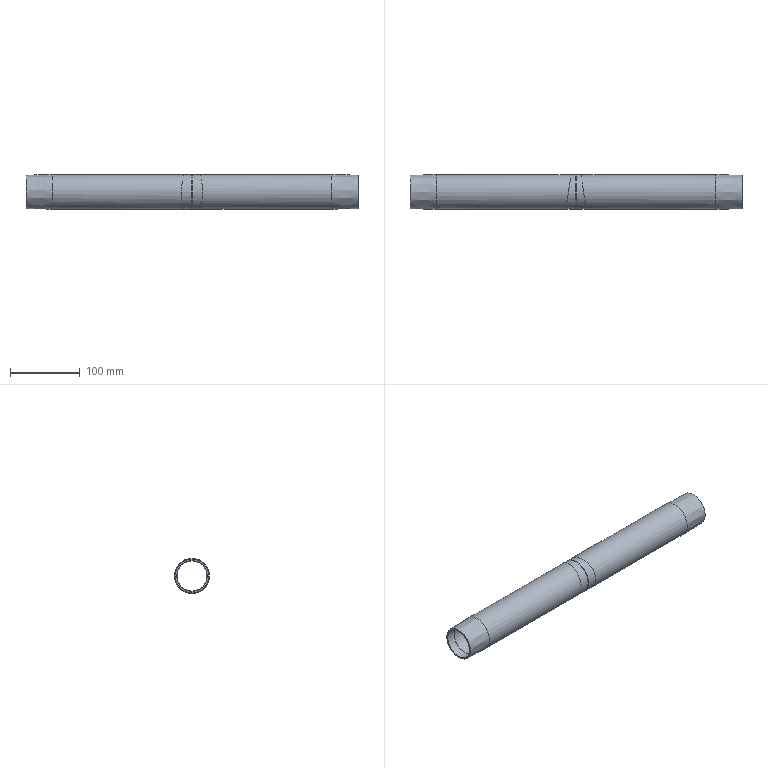Part | STEP file | 6150801 | 1 solid | 14 faces | box 475 x 50 x 50 mm | volume 235448 mm3 | cylinder 8 | plane 4 | cone 2 | commonest cylinder face diameters 50 x5 44 x2 43 x1
STEP:
#1=CARTESIAN_POINT('',(-0.5,-25.,0.));
#2=VERTEX_POINT('',#1);
#3=CARTESIAN_POINT('',(-0.5,0.,0.));
#4=DIRECTION('',(-1.,0.,0.));
#5=DIRECTION('',(0.,-1.,0.));
#6=AXIS2_PLACEMENT_3D('',#3,#4,#5);
#7=CIRCLE('',#6,25.);
#8=EDGE_CURVE('',#2,#2,#7,.T.);
#9=ORIENTED_EDGE('',*,*,#8,.F.);
#10=EDGE_LOOP('',(#9));
#11=FACE_OUTER_BOUND('',#10,.T.);
#12=CARTESIAN_POINT('',(0.5,25.,0.));
#13=VERTEX_POINT('',#12);
#14=CARTESIAN_POINT('',(0.5,0.,0.));
#15=DIRECTION('',(1.,0.,0.));
#16=DIRECTION('',(0.,1.,0.));
#17=AXIS2_PLACEMENT_3D('',#14,#15,#16);
#18=CIRCLE('',#17,25.);
#19=EDGE_CURVE('',#13,#13,#18,.T.);
#20=ORIENTED_EDGE('',*,*,#19,.F.);
#21=EDGE_LOOP('',(#20));
#22=FACE_OUTER_BOUND('',#21,.T.);
#23=CARTESIAN_POINT('',(-73.378,0.,0.));
#24=DIRECTION('',(-1.,0.,0.));
#25=DIRECTION('',(0.,0.,1.));
#26=AXIS2_PLACEMENT_3D('',#23,#24,#25);
#27=CYLINDRICAL_SURFACE('',#26,25.);
#28=ADVANCED_FACE('',(#11,#22),#27,.T.);
#29=CARTESIAN_POINT('',(200.,0.,25.));
#30=VERTEX_POINT('',#29);
#31=CARTESIAN_POINT('',(200.,0.,0.));
#32=DIRECTION('',(-1.,0.,0.));
#33=DIRECTION('',(0.,0.,1.));
#34=AXIS2_PLACEMENT_3D('',#31,#32,#33);
#35=CIRCLE('',#34,25.);
#36=EDGE_CURVE('',#30,#30,#35,.T.);
#37=ORIENTED_EDGE('',*,*,#36,.T.);
#38=EDGE_LOOP('',(#37));
#39=FACE_OUTER_BOUND('',#38,.T.);
#40=CARTESIAN_POINT('',(7.038,25.,0.));
#41=VERTEX_POINT('',#40);
#42=CARTESIAN_POINT('',(7.038,25.,0.));
#43=CARTESIAN_POINT('',(7.038,25.,-50.));
#44=CARTESIAN_POINT('',(14.731,-25.,-50.));
#45=CARTESIAN_POINT('',(14.731,-25.,0.));
#46=CARTESIAN_POINT('',(14.731,-25.,50.));
#47=CARTESIAN_POINT('',(7.038,25.,50.));
#48=CARTESIAN_POINT('',(7.038,25.,0.));
#49=(BOUNDED_CURVE()B_SPLINE_CURVE(3,(#42,#43,#44,#45,#46,#47,#48),.UNSPECIFIED.,.T.,.T.)B_SPLINE_CURVE_WITH_KNOTS((4,3,4),(0.,3.142,6.283),.UNSPECIFIED.)CURVE()GEOMETRIC_REPRESENTATION_ITEM()RATIONAL_B_SPLINE_CURVE((1.,0.3333,0.3333,1.,0.3333,0.3333,1.))REPRESENTATION_ITEM(''));
#50=EDGE_CURVE('',#41,#41,#49,.T.);
#51=ORIENTED_EDGE('',*,*,#50,.F.);
#52=EDGE_LOOP('',(#51));
#53=FACE_OUTER_BOUND('',#52,.T.);
#54=CARTESIAN_POINT('',(-73.378,0.,0.));
#55=DIRECTION('',(-1.,0.,0.));
#56=DIRECTION('',(0.,0.,1.));
#57=AXIS2_PLACEMENT_3D('',#54,#55,#56);
#58=CYLINDRICAL_SURFACE('',#57,25.);
#59=ADVANCED_FACE('',(#39,#53),#58,.T.);
#60=CARTESIAN_POINT('',(-200.,0.,25.));
#61=VERTEX_POINT('',#60);
#62=CARTESIAN_POINT('',(-200.,0.,0.));
#63=DIRECTION('',(-1.,0.,0.));
#64=DIRECTION('',(0.,0.,1.));
#65=AXIS2_PLACEMENT_3D('',#62,#63,#64);
#66=CIRCLE('',#65,25.);
#67=EDGE_CURVE('',#61,#61,#66,.T.);
#68=ORIENTED_EDGE('',*,*,#67,.F.);
#69=EDGE_LOOP('',(#68));
#70=FACE_OUTER_BOUND('',#69,.T.);
#71=CARTESIAN_POINT('',(-14.731,-25.,0.));
#72=VERTEX_POINT('',#71);
#73=CARTESIAN_POINT('',(-14.731,-25.,0.));
#74=CARTESIAN_POINT('',(-14.731,-25.,-50.));
#75=CARTESIAN_POINT('',(-7.038,25.,-50.));
#76=CARTESIAN_POINT('',(-7.038,25.,0.));
#77=CARTESIAN_POINT('',(-7.038,25.,50.));
#78=CARTESIAN_POINT('',(-14.731,-25.,50.));
#79=CARTESIAN_POINT('',(-14.731,-25.,0.));
#80=(BOUNDED_CURVE()B_SPLINE_CURVE(3,(#73,#74,#75,#76,#77,#78,#79),.UNSPECIFIED.,.T.,.F.)B_SPLINE_CURVE_WITH_KNOTS((4,3,4),(0.,3.142,6.283),.UNSPECIFIED.)CURVE()GEOMETRIC_REPRESENTATION_ITEM()RATIONAL_B_SPLINE_CURVE((1.,0.3333,0.3333,1.,0.3333,0.3333,1.))REPRESENTATION_ITEM(''));
#81=EDGE_CURVE('',#72,#72,#80,.T.);
#82=ORIENTED_EDGE('',*,*,#81,.F.);
#83=EDGE_LOOP('',(#82));
#84=FACE_OUTER_BOUND('',#83,.T.);
#85=CARTESIAN_POINT('',(-73.378,0.,0.));
#86=DIRECTION('',(-1.,0.,0.));
#87=DIRECTION('',(0.,0.,1.));
#88=AXIS2_PLACEMENT_3D('',#85,#86,#87);
#89=CYLINDRICAL_SURFACE('',#88,25.);
#90=ADVANCED_FACE('',(#70,#84),#89,.T.);
#91=ORIENTED_EDGE('',*,*,#19,.T.);
#92=EDGE_LOOP('',(#91));
#93=FACE_OUTER_BOUND('',#92,.T.);
#94=ORIENTED_EDGE('',*,*,#50,.T.);
#95=EDGE_LOOP('',(#94));
#96=FACE_OUTER_BOUND('',#95,.T.);
#97=CARTESIAN_POINT('',(-73.378,0.,0.));
#98=DIRECTION('',(-1.,0.,0.));
#99=DIRECTION('',(0.,0.,1.));
#100=AXIS2_PLACEMENT_3D('',#97,#98,#99);
#101=CYLINDRICAL_SURFACE('',#100,25.);
#102=ADVANCED_FACE('',(#93,#96),#101,.T.);
#103=CARTESIAN_POINT('',(237.5,0.,24.018));
#104=VERTEX_POINT('',#103);
#105=CARTESIAN_POINT('',(237.5,0.,0.));
#106=DIRECTION('',(-1.,0.,0.));
#107=DIRECTION('',(0.,0.,1.));
#108=AXIS2_PLACEMENT_3D('',#105,#106,#107);
#109=CIRCLE('',#108,24.018);
#110=EDGE_CURVE('',#104,#104,#109,.T.);
#111=ORIENTED_EDGE('',*,*,#110,.F.);
#112=EDGE_LOOP('',(#111));
#113=FACE_OUTER_BOUND('',#112,.T.);
#114=CARTESIAN_POINT('',(237.5,0.,22.));
#115=VERTEX_POINT('',#114);
#116=CARTESIAN_POINT('',(237.5,0.,0.));
#117=DIRECTION('',(-1.,0.,0.));
#118=DIRECTION('',(0.,0.,1.));
#119=AXIS2_PLACEMENT_3D('',#116,#117,#118);
#120=CIRCLE('',#119,22.);
#121=EDGE_CURVE('',#115,#115,#120,.T.);
#122=ORIENTED_EDGE('',*,*,#121,.T.);
#123=EDGE_LOOP('',(#122));
#124=FACE_BOUND('',#123,.T.);
#125=CARTESIAN_POINT('',(237.5,24.018,0.));
#126=DIRECTION('',(-1.,0.,0.));
#127=DIRECTION('',(0.,0.,1.));
#128=AXIS2_PLACEMENT_3D('',#125,#126,#127);
#129=PLANE('',#128);
#130=ADVANCED_FACE('',(#113,#124),#129,.F.);
#131=ORIENTED_EDGE('',*,*,#121,.F.);
#132=EDGE_LOOP('',(#131));
#133=FACE_OUTER_BOUND('',#132,.T.);
#134=CARTESIAN_POINT('',(225.,0.,22.));
#135=VERTEX_POINT('',#134);
#136=CARTESIAN_POINT('',(225.,0.,0.));
#137=DIRECTION('',(-1.,0.,0.));
#138=DIRECTION('',(0.,0.,1.));
#139=AXIS2_PLACEMENT_3D('',#136,#137,#138);
#140=CIRCLE('',#139,22.);
#141=EDGE_CURVE('',#135,#135,#140,.T.);
#142=ORIENTED_EDGE('',*,*,#141,.T.);
#143=EDGE_LOOP('',(#142));
#144=FACE_OUTER_BOUND('',#143,.T.);
#145=CARTESIAN_POINT('',(-73.378,0.,0.));
#146=DIRECTION('',(-1.,0.,0.));
#147=DIRECTION('',(0.,0.,1.));
#148=AXIS2_PLACEMENT_3D('',#145,#146,#147);
#149=CYLINDRICAL_SURFACE('',#148,22.);
#150=ADVANCED_FACE('',(#133,#144),#149,.F.);
#151=ORIENTED_EDGE('',*,*,#141,.F.);
#152=EDGE_LOOP('',(#151));
#153=FACE_OUTER_BOUND('',#152,.T.);
#154=CARTESIAN_POINT('',(225.,0.,21.5));
#155=VERTEX_POINT('',#154);
#156=CARTESIAN_POINT('',(225.,0.,0.));
#157=DIRECTION('',(-1.,0.,0.));
#158=DIRECTION('',(0.,0.,1.));
#159=AXIS2_PLACEMENT_3D('',#156,#157,#158);
#160=CIRCLE('',#159,21.5);
#161=EDGE_CURVE('',#155,#155,#160,.T.);
#162=ORIENTED_EDGE('',*,*,#161,.T.);
#163=EDGE_LOOP('',(#162));
#164=FACE_BOUND('',#163,.T.);
#165=CARTESIAN_POINT('',(225.,22.,0.));
#166=DIRECTION('',(-1.,0.,0.));
#167=DIRECTION('',(0.,0.,1.));
#168=AXIS2_PLACEMENT_3D('',#165,#166,#167);
#169=PLANE('',#168);
#170=ADVANCED_FACE('',(#153,#164),#169,.F.);
#171=ORIENTED_EDGE('',*,*,#161,.F.);
#172=EDGE_LOOP('',(#171));
#173=FACE_OUTER_BOUND('',#172,.T.);
#174=CARTESIAN_POINT('',(-225.,0.,21.5));
#175=VERTEX_POINT('',#174);
#176=CARTESIAN_POINT('',(-225.,0.,0.));
#177=DIRECTION('',(-1.,0.,0.));
#178=DIRECTION('',(0.,0.,1.));
#179=AXIS2_PLACEMENT_3D('',#176,#177,#178);
#180=CIRCLE('',#179,21.5);
#181=EDGE_CURVE('',#175,#175,#180,.T.);
#182=ORIENTED_EDGE('',*,*,#181,.T.);
#183=EDGE_LOOP('',(#182));
#184=FACE_OUTER_BOUND('',#183,.T.);
#185=CARTESIAN_POINT('',(-73.378,0.,0.));
#186=DIRECTION('',(-1.,0.,0.));
#187=DIRECTION('',(0.,0.,1.));
#188=AXIS2_PLACEMENT_3D('',#185,#186,#187);
#189=CYLINDRICAL_SURFACE('',#188,21.5);
#190=ADVANCED_FACE('',(#173,#184),#189,.F.);
#191=ORIENTED_EDGE('',*,*,#181,.F.);
#192=EDGE_LOOP('',(#191));
#193=FACE_BOUND('',#192,.T.);
#194=CARTESIAN_POINT('',(-225.,0.,22.));
#195=VERTEX_POINT('',#194);
#196=CARTESIAN_POINT('',(-225.,0.,0.));
#197=DIRECTION('',(-1.,0.,0.));
#198=DIRECTION('',(0.,0.,1.));
#199=AXIS2_PLACEMENT_3D('',#196,#197,#198);
#200=CIRCLE('',#199,22.);
#201=EDGE_CURVE('',#195,#195,#200,.T.);
#202=ORIENTED_EDGE('',*,*,#201,.T.);
#203=EDGE_LOOP('',(#202));
#204=FACE_OUTER_BOUND('',#203,.T.);
#205=CARTESIAN_POINT('',(-225.,22.,0.));
#206=DIRECTION('',(1.,0.,0.));
#207=DIRECTION('',(0.,0.,-1.));
#208=AXIS2_PLACEMENT_3D('',#205,#206,#207);
#209=PLANE('',#208);
#210=ADVANCED_FACE('',(#193,#204),#209,.F.);
#211=ORIENTED_EDGE('',*,*,#201,.F.);
#212=EDGE_LOOP('',(#211));
#213=FACE_OUTER_BOUND('',#212,.T.);
#214=CARTESIAN_POINT('',(-237.5,0.,22.));
#215=VERTEX_POINT('',#214);
#216=CARTESIAN_POINT('',(-237.5,0.,0.));
#217=DIRECTION('',(-1.,0.,0.));
#218=DIRECTION('',(0.,0.,1.));
#219=AXIS2_PLACEMENT_3D('',#216,#217,#218);
#220=CIRCLE('',#219,22.);
#221=EDGE_CURVE('',#215,#215,#220,.T.);
#222=ORIENTED_EDGE('',*,*,#221,.T.);
#223=EDGE_LOOP('',(#222));
#224=FACE_OUTER_BOUND('',#223,.T.);
#225=CARTESIAN_POINT('',(-73.378,0.,0.));
#226=DIRECTION('',(-1.,0.,0.));
#227=DIRECTION('',(0.,0.,1.));
#228=AXIS2_PLACEMENT_3D('',#225,#226,#227);
#229=CYLINDRICAL_SURFACE('',#228,22.);
#230=ADVANCED_FACE('',(#213,#224),#229,.F.);
#231=ORIENTED_EDGE('',*,*,#221,.F.);
#232=EDGE_LOOP('',(#231));
#233=FACE_BOUND('',#232,.T.);
#234=CARTESIAN_POINT('',(-237.5,0.,24.018));
#235=VERTEX_POINT('',#234);
#236=CARTESIAN_POINT('',(-237.5,0.,0.));
#237=DIRECTION('',(-1.,0.,0.));
#238=DIRECTION('',(0.,0.,1.));
#239=AXIS2_PLACEMENT_3D('',#236,#237,#238);
#240=CIRCLE('',#239,24.018);
#241=EDGE_CURVE('',#235,#235,#240,.T.);
#242=ORIENTED_EDGE('',*,*,#241,.T.);
#243=EDGE_LOOP('',(#242));
#244=FACE_OUTER_BOUND('',#243,.T.);
#245=CARTESIAN_POINT('',(-237.5,22.,0.));
#246=DIRECTION('',(1.,0.,0.));
#247=DIRECTION('',(0.,0.,-1.));
#248=AXIS2_PLACEMENT_3D('',#245,#246,#247);
#249=PLANE('',#248);
#250=ADVANCED_FACE('',(#233,#244),#249,.F.);
#251=ORIENTED_EDGE('',*,*,#241,.F.);
#252=EDGE_LOOP('',(#251));
#253=FACE_BOUND('',#252,.T.);
#254=ORIENTED_EDGE('',*,*,#67,.T.);
#255=EDGE_LOOP('',(#254));
#256=FACE_OUTER_BOUND('',#255,.T.);
#257=CARTESIAN_POINT('',(-200.,0.,0.));
#258=DIRECTION('',(1.,0.,0.));
#259=DIRECTION('',(0.,0.,-1.));
#260=AXIS2_PLACEMENT_3D('',#257,#258,#259);
#261=CONICAL_SURFACE('',#260,25.,0.02618);
#262=ADVANCED_FACE('',(#253,#256),#261,.T.);
#263=ORIENTED_EDGE('',*,*,#81,.T.);
#264=EDGE_LOOP('',(#263));
#265=FACE_OUTER_BOUND('',#264,.T.);
#266=ORIENTED_EDGE('',*,*,#8,.T.);
#267=EDGE_LOOP('',(#266));
#268=FACE_OUTER_BOUND('',#267,.T.);
#269=CARTESIAN_POINT('',(-73.378,0.,0.));
#270=DIRECTION('',(-1.,0.,0.));
#271=DIRECTION('',(0.,0.,1.));
#272=AXIS2_PLACEMENT_3D('',#269,#270,#271);
#273=CYLINDRICAL_SURFACE('',#272,25.);
#274=ADVANCED_FACE('',(#265,#268),#273,.T.);
#275=ORIENTED_EDGE('',*,*,#36,.F.);
#276=EDGE_LOOP('',(#275));
#277=FACE_OUTER_BOUND('',#276,.T.);
#278=ORIENTED_EDGE('',*,*,#110,.T.);
#279=EDGE_LOOP('',(#278));
#280=FACE_BOUND('',#279,.T.);
#281=CARTESIAN_POINT('',(237.5,0.,0.));
#282=DIRECTION('',(-1.,0.,0.));
#283=DIRECTION('',(0.,0.,1.));
#284=AXIS2_PLACEMENT_3D('',#281,#282,#283);
#285=CONICAL_SURFACE('',#284,24.018,0.02618);
#286=ADVANCED_FACE('',(#277,#280),#285,.T.);
#287=CLOSED_SHELL('',(#28,#59,#90,#102,#130,#150,#170,#190,#210,#230,#250,#262,#274,#286));
#288=MANIFOLD_SOLID_BREP('',#287);
#289=CARTESIAN_POINT('',(0.,0.,0.));
#290=DIRECTION('',(0.,0.,1.));
#291=DIRECTION('',(1.,0.,0.));
#292=AXIS2_PLACEMENT_3D('',#289,#290,#291);
#293=(LENGTH_UNIT()NAMED_UNIT(*)SI_UNIT(.MILLI.,.METRE.));
#294=UNCERTAINTY_MEASURE_WITH_UNIT(LENGTH_MEASURE(0.00001),#293,'','');
#295=(NAMED_UNIT(*)PLANE_ANGLE_UNIT()SI_UNIT($,.RADIAN.));
#296=(NAMED_UNIT(*)SI_UNIT($,.STERADIAN.)SOLID_ANGLE_UNIT());
#297=(GEOMETRIC_REPRESENTATION_CONTEXT(3)GLOBAL_UNCERTAINTY_ASSIGNED_CONTEXT((#294))GLOBAL_UNIT_ASSIGNED_CONTEXT((#293,#295,#296))REPRESENTATION_CONTEXT('',''));
#298=ADVANCED_BREP_SHAPE_REPRESENTATION('',(#288,#292),#297);